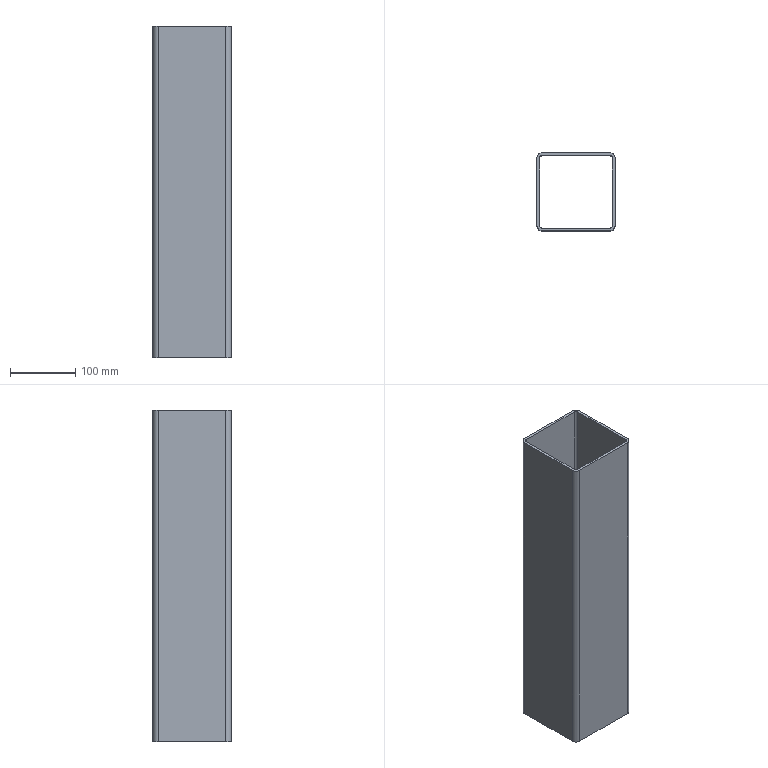Part | SolidWorks | features ICE 1, LibraryFeature 1 | 1 solid | 18 faces | box 120 x 120 x 510 mm | volume 925546 mm3 | plane 10 | cylinder 8 | commonest cylinder face diameters 8 x4 16 x4
STEP:
#1=CARTESIAN_POINT('',(52.,60.,-255.));
#2=VERTEX_POINT('',#1);
#3=CARTESIAN_POINT('',(-52.,60.,-255.));
#4=VERTEX_POINT('',#3);
#5=CARTESIAN_POINT('',(0.,60.,-255.));
#6=DIRECTION('',(-1.,0.,0.));
#7=VECTOR('',#6,1000.);
#8=LINE('',#5,#7);
#9=EDGE_CURVE('',#2,#4,#8,.T.);
#10=ORIENTED_EDGE('',*,*,#9,.T.);
#11=CARTESIAN_POINT('',(-52.,60.,255.));
#12=VERTEX_POINT('',#11);
#13=CARTESIAN_POINT('',(-52.,60.,255.));
#14=DIRECTION('',(0.,0.,-1.));
#15=VECTOR('',#14,1000.);
#16=LINE('',#13,#15);
#17=EDGE_CURVE('',#12,#4,#16,.T.);
#18=ORIENTED_EDGE('',*,*,#17,.F.);
#19=CARTESIAN_POINT('',(52.,60.,255.));
#20=VERTEX_POINT('',#19);
#21=CARTESIAN_POINT('',(0.,60.,255.));
#22=DIRECTION('',(-1.,0.,0.));
#23=VECTOR('',#22,1000.);
#24=LINE('',#21,#23);
#25=EDGE_CURVE('',#20,#12,#24,.T.);
#26=ORIENTED_EDGE('',*,*,#25,.F.);
#27=CARTESIAN_POINT('',(52.,60.,255.));
#28=DIRECTION('',(0.,0.,-1.));
#29=VECTOR('',#28,1000.);
#30=LINE('',#27,#29);
#31=EDGE_CURVE('',#20,#2,#30,.T.);
#32=ORIENTED_EDGE('',*,*,#31,.T.);
#33=EDGE_LOOP('',(#10,#18,#26,#32));
#34=FACE_OUTER_BOUND('',#33,.T.);
#35=CARTESIAN_POINT('',(0.,60.,255.));
#36=DIRECTION('',(0.,-1.,0.));
#37=DIRECTION('',(0.,0.,-1.));
#38=AXIS2_PLACEMENT_3D('',#35,#36,#37);
#39=PLANE('',#38);
#40=ADVANCED_FACE('',(#34),#39,.F.);
#41=CARTESIAN_POINT('',(-60.,52.,-255.));
#42=VERTEX_POINT('',#41);
#43=CARTESIAN_POINT('',(-52.,52.,-255.));
#44=DIRECTION('',(0.,0.,1.));
#45=DIRECTION('',(1.,0.,0.));
#46=AXIS2_PLACEMENT_3D('',#43,#44,#45);
#47=CIRCLE('',#46,8.);
#48=EDGE_CURVE('',#4,#42,#47,.T.);
#49=ORIENTED_EDGE('',*,*,#48,.T.);
#50=CARTESIAN_POINT('',(-60.,52.,255.));
#51=VERTEX_POINT('',#50);
#52=CARTESIAN_POINT('',(-60.,52.,255.));
#53=DIRECTION('',(0.,0.,-1.));
#54=VECTOR('',#53,1000.);
#55=LINE('',#52,#54);
#56=EDGE_CURVE('',#51,#42,#55,.T.);
#57=ORIENTED_EDGE('',*,*,#56,.F.);
#58=CARTESIAN_POINT('',(-52.,52.,255.));
#59=DIRECTION('',(0.,0.,1.));
#60=DIRECTION('',(1.,0.,0.));
#61=AXIS2_PLACEMENT_3D('',#58,#59,#60);
#62=CIRCLE('',#61,8.);
#63=EDGE_CURVE('',#12,#51,#62,.T.);
#64=ORIENTED_EDGE('',*,*,#63,.F.);
#65=ORIENTED_EDGE('',*,*,#17,.T.);
#66=EDGE_LOOP('',(#49,#57,#64,#65));
#67=FACE_OUTER_BOUND('',#66,.T.);
#68=CARTESIAN_POINT('',(-52.,52.,255.));
#69=DIRECTION('',(0.,0.,-1.));
#70=DIRECTION('',(-1.,0.,0.));
#71=AXIS2_PLACEMENT_3D('',#68,#69,#70);
#72=CYLINDRICAL_SURFACE('',#71,8.);
#73=ADVANCED_FACE('',(#67),#72,.T.);
#74=CARTESIAN_POINT('',(-60.,-52.,-255.));
#75=VERTEX_POINT('',#74);
#76=CARTESIAN_POINT('',(-60.,0.,-255.));
#77=DIRECTION('',(0.,1.,0.));
#78=VECTOR('',#77,1000.);
#79=LINE('',#76,#78);
#80=EDGE_CURVE('',#75,#42,#79,.T.);
#81=ORIENTED_EDGE('',*,*,#80,.F.);
#82=CARTESIAN_POINT('',(-60.,-52.,255.));
#83=VERTEX_POINT('',#82);
#84=CARTESIAN_POINT('',(-60.,-52.,255.));
#85=DIRECTION('',(0.,0.,-1.));
#86=VECTOR('',#85,1000.);
#87=LINE('',#84,#86);
#88=EDGE_CURVE('',#83,#75,#87,.T.);
#89=ORIENTED_EDGE('',*,*,#88,.F.);
#90=CARTESIAN_POINT('',(-60.,0.,255.));
#91=DIRECTION('',(0.,1.,0.));
#92=VECTOR('',#91,1000.);
#93=LINE('',#90,#92);
#94=EDGE_CURVE('',#83,#51,#93,.T.);
#95=ORIENTED_EDGE('',*,*,#94,.T.);
#96=ORIENTED_EDGE('',*,*,#56,.T.);
#97=EDGE_LOOP('',(#81,#89,#95,#96));
#98=FACE_OUTER_BOUND('',#97,.T.);
#99=CARTESIAN_POINT('',(-60.,0.,255.));
#100=DIRECTION('',(-1.,0.,0.));
#101=DIRECTION('',(0.,0.,1.));
#102=AXIS2_PLACEMENT_3D('',#99,#100,#101);
#103=PLANE('',#102);
#104=ADVANCED_FACE('',(#98),#103,.T.);
#105=CARTESIAN_POINT('',(-52.,-60.,-255.));
#106=VERTEX_POINT('',#105);
#107=CARTESIAN_POINT('',(-52.,-52.,-255.));
#108=DIRECTION('',(0.,0.,1.));
#109=DIRECTION('',(1.,0.,0.));
#110=AXIS2_PLACEMENT_3D('',#107,#108,#109);
#111=CIRCLE('',#110,8.);
#112=EDGE_CURVE('',#75,#106,#111,.T.);
#113=ORIENTED_EDGE('',*,*,#112,.T.);
#114=CARTESIAN_POINT('',(-52.,-60.,255.));
#115=VERTEX_POINT('',#114);
#116=CARTESIAN_POINT('',(-52.,-60.,255.));
#117=DIRECTION('',(0.,0.,-1.));
#118=VECTOR('',#117,1000.);
#119=LINE('',#116,#118);
#120=EDGE_CURVE('',#115,#106,#119,.T.);
#121=ORIENTED_EDGE('',*,*,#120,.F.);
#122=CARTESIAN_POINT('',(-52.,-52.,255.));
#123=DIRECTION('',(0.,0.,1.));
#124=DIRECTION('',(1.,0.,0.));
#125=AXIS2_PLACEMENT_3D('',#122,#123,#124);
#126=CIRCLE('',#125,8.);
#127=EDGE_CURVE('',#83,#115,#126,.T.);
#128=ORIENTED_EDGE('',*,*,#127,.F.);
#129=ORIENTED_EDGE('',*,*,#88,.T.);
#130=EDGE_LOOP('',(#113,#121,#128,#129));
#131=FACE_OUTER_BOUND('',#130,.T.);
#132=CARTESIAN_POINT('',(-52.,-52.,255.));
#133=DIRECTION('',(0.,0.,-1.));
#134=DIRECTION('',(-1.,0.,0.));
#135=AXIS2_PLACEMENT_3D('',#132,#133,#134);
#136=CYLINDRICAL_SURFACE('',#135,8.);
#137=ADVANCED_FACE('',(#131),#136,.T.);
#138=CARTESIAN_POINT('',(52.,-60.,-255.));
#139=VERTEX_POINT('',#138);
#140=CARTESIAN_POINT('',(0.,-60.,-255.));
#141=DIRECTION('',(1.,0.,0.));
#142=VECTOR('',#141,1000.);
#143=LINE('',#140,#142);
#144=EDGE_CURVE('',#106,#139,#143,.T.);
#145=ORIENTED_EDGE('',*,*,#144,.T.);
#146=CARTESIAN_POINT('',(52.,-60.,255.));
#147=VERTEX_POINT('',#146);
#148=CARTESIAN_POINT('',(52.,-60.,255.));
#149=DIRECTION('',(0.,0.,-1.));
#150=VECTOR('',#149,1000.);
#151=LINE('',#148,#150);
#152=EDGE_CURVE('',#147,#139,#151,.T.);
#153=ORIENTED_EDGE('',*,*,#152,.F.);
#154=CARTESIAN_POINT('',(0.,-60.,255.));
#155=DIRECTION('',(1.,0.,0.));
#156=VECTOR('',#155,1000.);
#157=LINE('',#154,#156);
#158=EDGE_CURVE('',#115,#147,#157,.T.);
#159=ORIENTED_EDGE('',*,*,#158,.F.);
#160=ORIENTED_EDGE('',*,*,#120,.T.);
#161=EDGE_LOOP('',(#145,#153,#159,#160));
#162=FACE_OUTER_BOUND('',#161,.T.);
#163=CARTESIAN_POINT('',(0.,-60.,255.));
#164=DIRECTION('',(0.,1.,0.));
#165=DIRECTION('',(0.,0.,1.));
#166=AXIS2_PLACEMENT_3D('',#163,#164,#165);
#167=PLANE('',#166);
#168=ADVANCED_FACE('',(#162),#167,.F.);
#169=CARTESIAN_POINT('',(60.,-52.,-255.));
#170=VERTEX_POINT('',#169);
#171=CARTESIAN_POINT('',(52.,-52.,-255.));
#172=DIRECTION('',(0.,0.,1.));
#173=DIRECTION('',(1.,0.,0.));
#174=AXIS2_PLACEMENT_3D('',#171,#172,#173);
#175=CIRCLE('',#174,8.);
#176=EDGE_CURVE('',#139,#170,#175,.T.);
#177=ORIENTED_EDGE('',*,*,#176,.T.);
#178=CARTESIAN_POINT('',(60.,-52.,255.));
#179=VERTEX_POINT('',#178);
#180=CARTESIAN_POINT('',(60.,-52.,255.));
#181=DIRECTION('',(0.,0.,-1.));
#182=VECTOR('',#181,1000.);
#183=LINE('',#180,#182);
#184=EDGE_CURVE('',#179,#170,#183,.T.);
#185=ORIENTED_EDGE('',*,*,#184,.F.);
#186=CARTESIAN_POINT('',(52.,-52.,255.));
#187=DIRECTION('',(0.,0.,1.));
#188=DIRECTION('',(1.,0.,0.));
#189=AXIS2_PLACEMENT_3D('',#186,#187,#188);
#190=CIRCLE('',#189,8.);
#191=EDGE_CURVE('',#147,#179,#190,.T.);
#192=ORIENTED_EDGE('',*,*,#191,.F.);
#193=ORIENTED_EDGE('',*,*,#152,.T.);
#194=EDGE_LOOP('',(#177,#185,#192,#193));
#195=FACE_OUTER_BOUND('',#194,.T.);
#196=CARTESIAN_POINT('',(52.,-52.,255.));
#197=DIRECTION('',(0.,0.,-1.));
#198=DIRECTION('',(-1.,0.,0.));
#199=AXIS2_PLACEMENT_3D('',#196,#197,#198);
#200=CYLINDRICAL_SURFACE('',#199,8.);
#201=ADVANCED_FACE('',(#195),#200,.T.);
#202=CARTESIAN_POINT('',(60.,52.,-255.));
#203=VERTEX_POINT('',#202);
#204=CARTESIAN_POINT('',(60.,0.,-255.));
#205=DIRECTION('',(0.,-1.,0.));
#206=VECTOR('',#205,1000.);
#207=LINE('',#204,#206);
#208=EDGE_CURVE('',#203,#170,#207,.T.);
#209=ORIENTED_EDGE('',*,*,#208,.F.);
#210=CARTESIAN_POINT('',(60.,52.,255.));
#211=VERTEX_POINT('',#210);
#212=CARTESIAN_POINT('',(60.,52.,255.));
#213=DIRECTION('',(0.,0.,-1.));
#214=VECTOR('',#213,1000.);
#215=LINE('',#212,#214);
#216=EDGE_CURVE('',#211,#203,#215,.T.);
#217=ORIENTED_EDGE('',*,*,#216,.F.);
#218=CARTESIAN_POINT('',(60.,0.,255.));
#219=DIRECTION('',(0.,-1.,0.));
#220=VECTOR('',#219,1000.);
#221=LINE('',#218,#220);
#222=EDGE_CURVE('',#211,#179,#221,.T.);
#223=ORIENTED_EDGE('',*,*,#222,.T.);
#224=ORIENTED_EDGE('',*,*,#184,.T.);
#225=EDGE_LOOP('',(#209,#217,#223,#224));
#226=FACE_OUTER_BOUND('',#225,.T.);
#227=CARTESIAN_POINT('',(60.,0.,255.));
#228=DIRECTION('',(1.,0.,0.));
#229=DIRECTION('',(0.,0.,-1.));
#230=AXIS2_PLACEMENT_3D('',#227,#228,#229);
#231=PLANE('',#230);
#232=ADVANCED_FACE('',(#226),#231,.T.);
#233=CARTESIAN_POINT('',(-56.,-52.,-255.));
#234=VERTEX_POINT('',#233);
#235=CARTESIAN_POINT('',(-52.,-56.,-255.));
#236=VERTEX_POINT('',#235);
#237=CARTESIAN_POINT('',(-52.,-52.,-255.));
#238=DIRECTION('',(0.,0.,1.));
#239=DIRECTION('',(1.,0.,0.));
#240=AXIS2_PLACEMENT_3D('',#237,#238,#239);
#241=CIRCLE('',#240,4.);
#242=EDGE_CURVE('',#234,#236,#241,.T.);
#243=ORIENTED_EDGE('',*,*,#242,.F.);
#244=CARTESIAN_POINT('',(-56.,-52.,255.));
#245=VERTEX_POINT('',#244);
#246=CARTESIAN_POINT('',(-56.,-52.,255.));
#247=DIRECTION('',(0.,0.,-1.));
#248=VECTOR('',#247,1000.);
#249=LINE('',#246,#248);
#250=EDGE_CURVE('',#245,#234,#249,.T.);
#251=ORIENTED_EDGE('',*,*,#250,.F.);
#252=CARTESIAN_POINT('',(-52.,-56.,255.));
#253=VERTEX_POINT('',#252);
#254=CARTESIAN_POINT('',(-52.,-52.,255.));
#255=DIRECTION('',(0.,0.,1.));
#256=DIRECTION('',(1.,0.,0.));
#257=AXIS2_PLACEMENT_3D('',#254,#255,#256);
#258=CIRCLE('',#257,4.);
#259=EDGE_CURVE('',#245,#253,#258,.T.);
#260=ORIENTED_EDGE('',*,*,#259,.T.);
#261=CARTESIAN_POINT('',(-52.,-56.,255.));
#262=DIRECTION('',(0.,0.,-1.));
#263=VECTOR('',#262,1000.);
#264=LINE('',#261,#263);
#265=EDGE_CURVE('',#253,#236,#264,.T.);
#266=ORIENTED_EDGE('',*,*,#265,.T.);
#267=EDGE_LOOP('',(#243,#251,#260,#266));
#268=FACE_OUTER_BOUND('',#267,.T.);
#269=CARTESIAN_POINT('',(-52.,-52.,255.));
#270=DIRECTION('',(0.,0.,-1.));
#271=DIRECTION('',(-1.,0.,0.));
#272=AXIS2_PLACEMENT_3D('',#269,#270,#271);
#273=CYLINDRICAL_SURFACE('',#272,4.);
#274=ADVANCED_FACE('',(#268),#273,.F.);
#275=CARTESIAN_POINT('',(-56.,52.,-255.));
#276=VERTEX_POINT('',#275);
#277=CARTESIAN_POINT('',(-56.,0.,-255.));
#278=DIRECTION('',(0.,1.,0.));
#279=VECTOR('',#278,1000.);
#280=LINE('',#277,#279);
#281=EDGE_CURVE('',#234,#276,#280,.T.);
#282=ORIENTED_EDGE('',*,*,#281,.T.);
#283=CARTESIAN_POINT('',(-56.,52.,255.));
#284=VERTEX_POINT('',#283);
#285=CARTESIAN_POINT('',(-56.,52.,255.));
#286=DIRECTION('',(0.,0.,-1.));
#287=VECTOR('',#286,1000.);
#288=LINE('',#285,#287);
#289=EDGE_CURVE('',#284,#276,#288,.T.);
#290=ORIENTED_EDGE('',*,*,#289,.F.);
#291=CARTESIAN_POINT('',(-56.,0.,255.));
#292=DIRECTION('',(0.,1.,0.));
#293=VECTOR('',#292,1000.);
#294=LINE('',#291,#293);
#295=EDGE_CURVE('',#245,#284,#294,.T.);
#296=ORIENTED_EDGE('',*,*,#295,.F.);
#297=ORIENTED_EDGE('',*,*,#250,.T.);
#298=EDGE_LOOP('',(#282,#290,#296,#297));
#299=FACE_OUTER_BOUND('',#298,.T.);
#300=CARTESIAN_POINT('',(-56.,0.,255.));
#301=DIRECTION('',(-1.,0.,0.));
#302=DIRECTION('',(0.,0.,1.));
#303=AXIS2_PLACEMENT_3D('',#300,#301,#302);
#304=PLANE('',#303);
#305=ADVANCED_FACE('',(#299),#304,.F.);
#306=CARTESIAN_POINT('',(-52.,56.,-255.));
#307=VERTEX_POINT('',#306);
#308=CARTESIAN_POINT('',(-52.,52.,-255.));
#309=DIRECTION('',(0.,0.,1.));
#310=DIRECTION('',(1.,0.,0.));
#311=AXIS2_PLACEMENT_3D('',#308,#309,#310);
#312=CIRCLE('',#311,4.);
#313=EDGE_CURVE('',#307,#276,#312,.T.);
#314=ORIENTED_EDGE('',*,*,#313,.F.);
#315=CARTESIAN_POINT('',(-52.,56.,255.));
#316=VERTEX_POINT('',#315);
#317=CARTESIAN_POINT('',(-52.,56.,255.));
#318=DIRECTION('',(0.,0.,-1.));
#319=VECTOR('',#318,1000.);
#320=LINE('',#317,#319);
#321=EDGE_CURVE('',#316,#307,#320,.T.);
#322=ORIENTED_EDGE('',*,*,#321,.F.);
#323=CARTESIAN_POINT('',(-52.,52.,255.));
#324=DIRECTION('',(0.,0.,1.));
#325=DIRECTION('',(1.,0.,0.));
#326=AXIS2_PLACEMENT_3D('',#323,#324,#325);
#327=CIRCLE('',#326,4.);
#328=EDGE_CURVE('',#316,#284,#327,.T.);
#329=ORIENTED_EDGE('',*,*,#328,.T.);
#330=ORIENTED_EDGE('',*,*,#289,.T.);
#331=EDGE_LOOP('',(#314,#322,#329,#330));
#332=FACE_OUTER_BOUND('',#331,.T.);
#333=CARTESIAN_POINT('',(-52.,52.,255.));
#334=DIRECTION('',(0.,0.,-1.));
#335=DIRECTION('',(-1.,0.,0.));
#336=AXIS2_PLACEMENT_3D('',#333,#334,#335);
#337=CYLINDRICAL_SURFACE('',#336,4.);
#338=ADVANCED_FACE('',(#332),#337,.F.);
#339=CARTESIAN_POINT('',(52.,56.,-255.));
#340=VERTEX_POINT('',#339);
#341=CARTESIAN_POINT('',(0.,56.,-255.));
#342=DIRECTION('',(-1.,0.,0.));
#343=VECTOR('',#342,1000.);
#344=LINE('',#341,#343);
#345=EDGE_CURVE('',#340,#307,#344,.T.);
#346=ORIENTED_EDGE('',*,*,#345,.F.);
#347=CARTESIAN_POINT('',(52.,56.,255.));
#348=VERTEX_POINT('',#347);
#349=CARTESIAN_POINT('',(52.,56.,255.));
#350=DIRECTION('',(0.,0.,-1.));
#351=VECTOR('',#350,1000.);
#352=LINE('',#349,#351);
#353=EDGE_CURVE('',#348,#340,#352,.T.);
#354=ORIENTED_EDGE('',*,*,#353,.F.);
#355=CARTESIAN_POINT('',(0.,56.,255.));
#356=DIRECTION('',(-1.,0.,0.));
#357=VECTOR('',#356,1000.);
#358=LINE('',#355,#357);
#359=EDGE_CURVE('',#348,#316,#358,.T.);
#360=ORIENTED_EDGE('',*,*,#359,.T.);
#361=ORIENTED_EDGE('',*,*,#321,.T.);
#362=EDGE_LOOP('',(#346,#354,#360,#361));
#363=FACE_OUTER_BOUND('',#362,.T.);
#364=CARTESIAN_POINT('',(0.,56.,255.));
#365=DIRECTION('',(0.,-1.,0.));
#366=DIRECTION('',(0.,0.,-1.));
#367=AXIS2_PLACEMENT_3D('',#364,#365,#366);
#368=PLANE('',#367);
#369=ADVANCED_FACE('',(#363),#368,.T.);
#370=CARTESIAN_POINT('',(56.,52.,-255.));
#371=VERTEX_POINT('',#370);
#372=CARTESIAN_POINT('',(52.,52.,-255.));
#373=DIRECTION('',(0.,0.,1.));
#374=DIRECTION('',(1.,0.,0.));
#375=AXIS2_PLACEMENT_3D('',#372,#373,#374);
#376=CIRCLE('',#375,4.);
#377=EDGE_CURVE('',#371,#340,#376,.T.);
#378=ORIENTED_EDGE('',*,*,#377,.F.);
#379=CARTESIAN_POINT('',(56.,52.,255.));
#380=VERTEX_POINT('',#379);
#381=CARTESIAN_POINT('',(56.,52.,255.));
#382=DIRECTION('',(0.,0.,-1.));
#383=VECTOR('',#382,1000.);
#384=LINE('',#381,#383);
#385=EDGE_CURVE('',#380,#371,#384,.T.);
#386=ORIENTED_EDGE('',*,*,#385,.F.);
#387=CARTESIAN_POINT('',(52.,52.,255.));
#388=DIRECTION('',(0.,0.,1.));
#389=DIRECTION('',(1.,0.,0.));
#390=AXIS2_PLACEMENT_3D('',#387,#388,#389);
#391=CIRCLE('',#390,4.);
#392=EDGE_CURVE('',#380,#348,#391,.T.);
#393=ORIENTED_EDGE('',*,*,#392,.T.);
#394=ORIENTED_EDGE('',*,*,#353,.T.);
#395=EDGE_LOOP('',(#378,#386,#393,#394));
#396=FACE_OUTER_BOUND('',#395,.T.);
#397=CARTESIAN_POINT('',(52.,52.,255.));
#398=DIRECTION('',(0.,0.,-1.));
#399=DIRECTION('',(-1.,0.,0.));
#400=AXIS2_PLACEMENT_3D('',#397,#398,#399);
#401=CYLINDRICAL_SURFACE('',#400,4.);
#402=ADVANCED_FACE('',(#396),#401,.F.);
#403=CARTESIAN_POINT('',(56.,-52.,-255.));
#404=VERTEX_POINT('',#403);
#405=CARTESIAN_POINT('',(56.,0.,-255.));
#406=DIRECTION('',(0.,-1.,0.));
#407=VECTOR('',#406,1000.);
#408=LINE('',#405,#407);
#409=EDGE_CURVE('',#371,#404,#408,.T.);
#410=ORIENTED_EDGE('',*,*,#409,.T.);
#411=CARTESIAN_POINT('',(56.,-52.,255.));
#412=VERTEX_POINT('',#411);
#413=CARTESIAN_POINT('',(56.,-52.,255.));
#414=DIRECTION('',(0.,0.,-1.));
#415=VECTOR('',#414,1000.);
#416=LINE('',#413,#415);
#417=EDGE_CURVE('',#412,#404,#416,.T.);
#418=ORIENTED_EDGE('',*,*,#417,.F.);
#419=CARTESIAN_POINT('',(56.,0.,255.));
#420=DIRECTION('',(0.,-1.,0.));
#421=VECTOR('',#420,1000.);
#422=LINE('',#419,#421);
#423=EDGE_CURVE('',#380,#412,#422,.T.);
#424=ORIENTED_EDGE('',*,*,#423,.F.);
#425=ORIENTED_EDGE('',*,*,#385,.T.);
#426=EDGE_LOOP('',(#410,#418,#424,#425));
#427=FACE_OUTER_BOUND('',#426,.T.);
#428=CARTESIAN_POINT('',(56.,0.,255.));
#429=DIRECTION('',(1.,0.,0.));
#430=DIRECTION('',(0.,0.,-1.));
#431=AXIS2_PLACEMENT_3D('',#428,#429,#430);
#432=PLANE('',#431);
#433=ADVANCED_FACE('',(#427),#432,.F.);
#434=CARTESIAN_POINT('',(52.,-56.,-255.));
#435=VERTEX_POINT('',#434);
#436=CARTESIAN_POINT('',(52.,-52.,-255.));
#437=DIRECTION('',(0.,0.,1.));
#438=DIRECTION('',(1.,0.,0.));
#439=AXIS2_PLACEMENT_3D('',#436,#437,#438);
#440=CIRCLE('',#439,4.);
#441=EDGE_CURVE('',#435,#404,#440,.T.);
#442=ORIENTED_EDGE('',*,*,#441,.F.);
#443=CARTESIAN_POINT('',(52.,-56.,255.));
#444=VERTEX_POINT('',#443);
#445=CARTESIAN_POINT('',(52.,-56.,255.));
#446=DIRECTION('',(0.,0.,-1.));
#447=VECTOR('',#446,1000.);
#448=LINE('',#445,#447);
#449=EDGE_CURVE('',#444,#435,#448,.T.);
#450=ORIENTED_EDGE('',*,*,#449,.F.);
#451=CARTESIAN_POINT('',(52.,-52.,255.));
#452=DIRECTION('',(0.,0.,1.));
#453=DIRECTION('',(1.,0.,0.));
#454=AXIS2_PLACEMENT_3D('',#451,#452,#453);
#455=CIRCLE('',#454,4.);
#456=EDGE_CURVE('',#444,#412,#455,.T.);
#457=ORIENTED_EDGE('',*,*,#456,.T.);
#458=ORIENTED_EDGE('',*,*,#417,.T.);
#459=EDGE_LOOP('',(#442,#450,#457,#458));
#460=FACE_OUTER_BOUND('',#459,.T.);
#461=CARTESIAN_POINT('',(52.,-52.,255.));
#462=DIRECTION('',(0.,0.,-1.));
#463=DIRECTION('',(-1.,0.,0.));
#464=AXIS2_PLACEMENT_3D('',#461,#462,#463);
#465=CYLINDRICAL_SURFACE('',#464,4.);
#466=ADVANCED_FACE('',(#460),#465,.F.);
#467=CARTESIAN_POINT('',(0.,-56.,-255.));
#468=DIRECTION('',(1.,0.,0.));
#469=VECTOR('',#468,1000.);
#470=LINE('',#467,#469);
#471=EDGE_CURVE('',#236,#435,#470,.T.);
#472=ORIENTED_EDGE('',*,*,#471,.F.);
#473=ORIENTED_EDGE('',*,*,#265,.F.);
#474=CARTESIAN_POINT('',(0.,-56.,255.));
#475=DIRECTION('',(1.,0.,0.));
#476=VECTOR('',#475,1000.);
#477=LINE('',#474,#476);
#478=EDGE_CURVE('',#253,#444,#477,.T.);
#479=ORIENTED_EDGE('',*,*,#478,.T.);
#480=ORIENTED_EDGE('',*,*,#449,.T.);
#481=EDGE_LOOP('',(#472,#473,#479,#480));
#482=FACE_OUTER_BOUND('',#481,.T.);
#483=CARTESIAN_POINT('',(0.,-56.,255.));
#484=DIRECTION('',(0.,1.,0.));
#485=DIRECTION('',(0.,0.,1.));
#486=AXIS2_PLACEMENT_3D('',#483,#484,#485);
#487=PLANE('',#486);
#488=ADVANCED_FACE('',(#482),#487,.T.);
#489=CARTESIAN_POINT('',(52.,52.,-255.));
#490=DIRECTION('',(0.,0.,1.));
#491=DIRECTION('',(1.,0.,0.));
#492=AXIS2_PLACEMENT_3D('',#489,#490,#491);
#493=CIRCLE('',#492,8.);
#494=EDGE_CURVE('',#203,#2,#493,.T.);
#495=ORIENTED_EDGE('',*,*,#494,.T.);
#496=ORIENTED_EDGE('',*,*,#31,.F.);
#497=CARTESIAN_POINT('',(52.,52.,255.));
#498=DIRECTION('',(0.,0.,1.));
#499=DIRECTION('',(1.,0.,0.));
#500=AXIS2_PLACEMENT_3D('',#497,#498,#499);
#501=CIRCLE('',#500,8.);
#502=EDGE_CURVE('',#211,#20,#501,.T.);
#503=ORIENTED_EDGE('',*,*,#502,.F.);
#504=ORIENTED_EDGE('',*,*,#216,.T.);
#505=EDGE_LOOP('',(#495,#496,#503,#504));
#506=FACE_OUTER_BOUND('',#505,.T.);
#507=CARTESIAN_POINT('',(52.,52.,255.));
#508=DIRECTION('',(0.,0.,-1.));
#509=DIRECTION('',(-1.,0.,0.));
#510=AXIS2_PLACEMENT_3D('',#507,#508,#509);
#511=CYLINDRICAL_SURFACE('',#510,8.);
#512=ADVANCED_FACE('',(#506),#511,.T.);
#513=ORIENTED_EDGE('',*,*,#259,.F.);
#514=ORIENTED_EDGE('',*,*,#295,.T.);
#515=ORIENTED_EDGE('',*,*,#328,.F.);
#516=ORIENTED_EDGE('',*,*,#359,.F.);
#517=ORIENTED_EDGE('',*,*,#392,.F.);
#518=ORIENTED_EDGE('',*,*,#423,.T.);
#519=ORIENTED_EDGE('',*,*,#456,.F.);
#520=ORIENTED_EDGE('',*,*,#478,.F.);
#521=EDGE_LOOP('',(#513,#514,#515,#516,#517,#518,#519,#520));
#522=FACE_BOUND('',#521,.T.);
#523=ORIENTED_EDGE('',*,*,#25,.T.);
#524=ORIENTED_EDGE('',*,*,#63,.T.);
#525=ORIENTED_EDGE('',*,*,#94,.F.);
#526=ORIENTED_EDGE('',*,*,#127,.T.);
#527=ORIENTED_EDGE('',*,*,#158,.T.);
#528=ORIENTED_EDGE('',*,*,#191,.T.);
#529=ORIENTED_EDGE('',*,*,#222,.F.);
#530=ORIENTED_EDGE('',*,*,#502,.T.);
#531=EDGE_LOOP('',(#523,#524,#525,#526,#527,#528,#529,#530));
#532=FACE_OUTER_BOUND('',#531,.T.);
#533=CARTESIAN_POINT('',(0.,0.,255.));
#534=DIRECTION('',(0.,0.,1.));
#535=DIRECTION('',(1.,0.,0.));
#536=AXIS2_PLACEMENT_3D('',#533,#534,#535);
#537=PLANE('',#536);
#538=ADVANCED_FACE('',(#522,#532),#537,.T.);
#539=ORIENTED_EDGE('',*,*,#242,.T.);
#540=ORIENTED_EDGE('',*,*,#471,.T.);
#541=ORIENTED_EDGE('',*,*,#441,.T.);
#542=ORIENTED_EDGE('',*,*,#409,.F.);
#543=ORIENTED_EDGE('',*,*,#377,.T.);
#544=ORIENTED_EDGE('',*,*,#345,.T.);
#545=ORIENTED_EDGE('',*,*,#313,.T.);
#546=ORIENTED_EDGE('',*,*,#281,.F.);
#547=EDGE_LOOP('',(#539,#540,#541,#542,#543,#544,#545,#546));
#548=FACE_BOUND('',#547,.T.);
#549=ORIENTED_EDGE('',*,*,#9,.F.);
#550=ORIENTED_EDGE('',*,*,#494,.F.);
#551=ORIENTED_EDGE('',*,*,#208,.T.);
#552=ORIENTED_EDGE('',*,*,#176,.F.);
#553=ORIENTED_EDGE('',*,*,#144,.F.);
#554=ORIENTED_EDGE('',*,*,#112,.F.);
#555=ORIENTED_EDGE('',*,*,#80,.T.);
#556=ORIENTED_EDGE('',*,*,#48,.F.);
#557=EDGE_LOOP('',(#549,#550,#551,#552,#553,#554,#555,#556));
#558=FACE_OUTER_BOUND('',#557,.T.);
#559=CARTESIAN_POINT('',(0.,0.,-255.));
#560=DIRECTION('',(0.,0.,1.));
#561=DIRECTION('',(1.,0.,0.));
#562=AXIS2_PLACEMENT_3D('',#559,#560,#561);
#563=PLANE('',#562);
#564=ADVANCED_FACE('',(#548,#558),#563,.F.);
#565=CLOSED_SHELL('',(#40,#73,#104,#137,#168,#201,#232,#274,#305,#338,#369,#402,#433,#466,#488,#512,#538,#564));
#566=MANIFOLD_SOLID_BREP('',#565);
#567=CARTESIAN_POINT('',(0.,0.,0.));
#568=DIRECTION('',(0.,0.,1.));
#569=DIRECTION('',(1.,0.,0.));
#570=AXIS2_PLACEMENT_3D('',#567,#568,#569);
#571=(LENGTH_UNIT()NAMED_UNIT(*)SI_UNIT(.MILLI.,.METRE.));
#572=UNCERTAINTY_MEASURE_WITH_UNIT(LENGTH_MEASURE(0.00001),#571,'','');
#573=(NAMED_UNIT(*)PLANE_ANGLE_UNIT()SI_UNIT($,.RADIAN.));
#574=(NAMED_UNIT(*)SI_UNIT($,.STERADIAN.)SOLID_ANGLE_UNIT());
#575=(GEOMETRIC_REPRESENTATION_CONTEXT(3)GLOBAL_UNCERTAINTY_ASSIGNED_CONTEXT((#572))GLOBAL_UNIT_ASSIGNED_CONTEXT((#571,#573,#574))REPRESENTATION_CONTEXT('',''));
#576=ADVANCED_BREP_SHAPE_REPRESENTATION('',(#566,#570),#575);